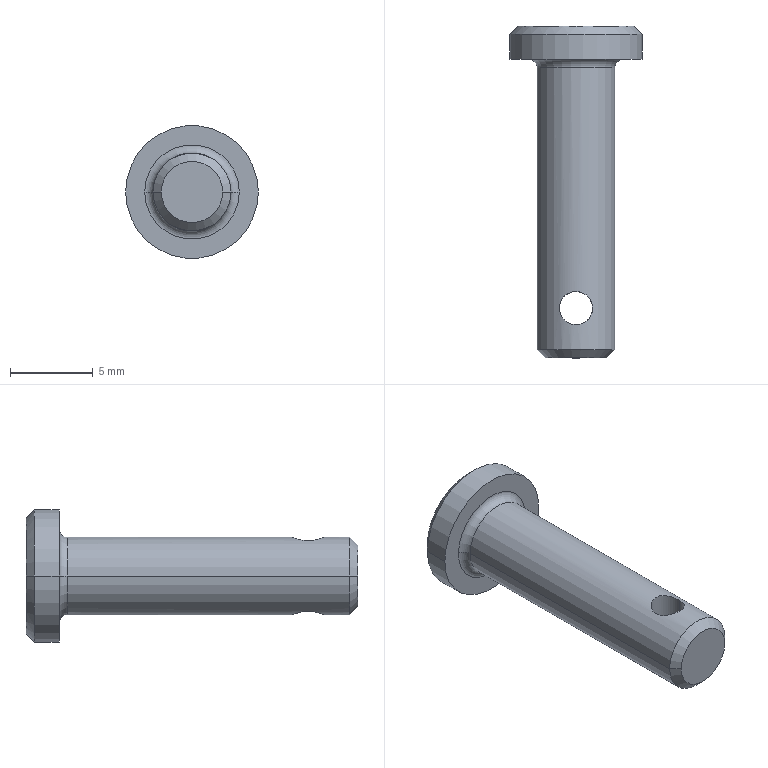Part | SolidWorks | features Chamfer 1, Fillet 1, ICE 1, Revolution 1 | 1 solid | 15 faces | box 8 x 20 x 8 mm | volume 394.503 mm3 | cylinder 6 | cone 4 | plane 3 | torus 2 | commonest cylinder face diameters 2 x2 4.7 x2 8 x2
STEP:
#1=CARTESIAN_POINT('',(1.,-17.,-2.127));
#2=VERTEX_POINT('',#1);
#3=CARTESIAN_POINT('',(-1.,-17.,-2.127));
#4=VERTEX_POINT('',#3);
#5=CARTESIAN_POINT('',(1.,-17.,-2.127));
#6=CARTESIAN_POINT('',(1.,-17.134,-2.127));
#7=CARTESIAN_POINT('',(0.9731,-17.265,-2.14));
#8=CARTESIAN_POINT('',(0.8722,-17.506,-2.183));
#9=CARTESIAN_POINT('',(0.7982,-17.616,-2.212));
#10=CARTESIAN_POINT('',(0.616,-17.798,-2.27));
#11=CARTESIAN_POINT('',(0.5058,-17.872,-2.298));
#12=CARTESIAN_POINT('',(0.2655,-17.973,-2.338));
#13=CARTESIAN_POINT('',(0.1329,-18.,-2.35));
#14=CARTESIAN_POINT('',(-0.1318,-18.,-2.35));
#15=CARTESIAN_POINT('',(-0.2639,-17.974,-2.338));
#16=CARTESIAN_POINT('',(-0.5076,-17.872,-2.298));
#17=CARTESIAN_POINT('',(-0.6167,-17.798,-2.27));
#18=CARTESIAN_POINT('',(-0.7992,-17.615,-2.212));
#19=CARTESIAN_POINT('',(-0.873,-17.505,-2.183));
#20=CARTESIAN_POINT('',(-0.973,-17.265,-2.14));
#21=CARTESIAN_POINT('',(-1.,-17.132,-2.127));
#22=CARTESIAN_POINT('',(-1.,-17.,-2.127));
#23=B_SPLINE_CURVE_WITH_KNOTS('',3,(#5,#6,#7,#8,#9,#10,#11,#12,#13,#14,#15,#16,#17,#18,#19,#20,#21,#22),.UNSPECIFIED.,.F.,.F.,(4,2,2,2,2,2,2,2,4),(0.,0.0003956,0.0007911,0.001187,0.001582,0.001978,0.002373,0.002769,0.003164),.UNSPECIFIED.);
#24=EDGE_CURVE('',#2,#4,#23,.T.);
#25=ORIENTED_EDGE('',*,*,#24,.T.);
#26=CARTESIAN_POINT('',(-1.,-17.,2.127));
#27=VERTEX_POINT('',#26);
#28=CARTESIAN_POINT('',(-1.,-17.,-4.));
#29=DIRECTION('',(0.,0.,1.));
#30=VECTOR('',#29,1000.);
#31=LINE('',#28,#30);
#32=EDGE_CURVE('',#4,#27,#31,.T.);
#33=ORIENTED_EDGE('',*,*,#32,.T.);
#34=CARTESIAN_POINT('',(1.,-17.,2.127));
#35=VERTEX_POINT('',#34);
#36=CARTESIAN_POINT('',(-1.,-17.,2.127));
#37=CARTESIAN_POINT('',(-1.,-17.132,2.127));
#38=CARTESIAN_POINT('',(-0.9733,-17.264,2.14));
#39=CARTESIAN_POINT('',(-0.8723,-17.506,2.183));
#40=CARTESIAN_POINT('',(-0.7988,-17.615,2.212));
#41=CARTESIAN_POINT('',(-0.6151,-17.799,2.27));
#42=CARTESIAN_POINT('',(-0.5058,-17.872,2.298));
#43=CARTESIAN_POINT('',(-0.2646,-17.973,2.338));
#44=CARTESIAN_POINT('',(-0.1321,-18.,2.35));
#45=CARTESIAN_POINT('',(0.1317,-18.,2.35));
#46=CARTESIAN_POINT('',(0.2646,-17.973,2.338));
#47=CARTESIAN_POINT('',(0.5058,-17.872,2.298));
#48=CARTESIAN_POINT('',(0.6155,-17.799,2.27));
#49=CARTESIAN_POINT('',(0.8909,-17.523,2.183));
#50=CARTESIAN_POINT('',(1.,-17.268,2.127));
#51=CARTESIAN_POINT('',(1.,-17.,2.127));
#52=B_SPLINE_CURVE_WITH_KNOTS('',3,(#36,#37,#38,#39,#40,#41,#42,#43,#44,#45,#46,#47,#48,#49,#50,#51),.UNSPECIFIED.,.F.,.F.,(4,2,2,2,2,2,2,4),(0.003164,0.00356,0.003955,0.00435,0.004745,0.00514,0.005536,0.006326),.UNSPECIFIED.);
#53=EDGE_CURVE('',#27,#35,#52,.T.);
#54=ORIENTED_EDGE('',*,*,#53,.T.);
#55=CARTESIAN_POINT('',(1.,-17.,-4.));
#56=DIRECTION('',(0.,0.,1.));
#57=VECTOR('',#56,1000.);
#58=LINE('',#55,#57);
#59=EDGE_CURVE('',#2,#35,#58,.T.);
#60=ORIENTED_EDGE('',*,*,#59,.F.);
#61=EDGE_LOOP('',(#25,#33,#54,#60));
#62=FACE_OUTER_BOUND('',#61,.T.);
#63=CARTESIAN_POINT('',(0.,-17.,-4.));
#64=DIRECTION('',(0.,0.,1.));
#65=DIRECTION('',(1.,0.,0.));
#66=AXIS2_PLACEMENT_3D('',#63,#64,#65);
#67=CYLINDRICAL_SURFACE('',#66,1.);
#68=ADVANCED_FACE('',(#62),#67,.F.);
#69=CARTESIAN_POINT('',(-3.5,0.,0.));
#70=VERTEX_POINT('',#69);
#71=CARTESIAN_POINT('',(3.5,0.,0.));
#72=VERTEX_POINT('',#71);
#73=CARTESIAN_POINT('',(0.,0.,0.));
#74=DIRECTION('',(0.,1.,0.));
#75=DIRECTION('',(-1.,0.,0.));
#76=AXIS2_PLACEMENT_3D('',#73,#74,#75);
#77=CIRCLE('',#76,3.5);
#78=EDGE_CURVE('',#70,#72,#77,.T.);
#79=ORIENTED_EDGE('',*,*,#78,.F.);
#80=CARTESIAN_POINT('',(-4.,-0.5,0.));
#81=VERTEX_POINT('',#80);
#82=CARTESIAN_POINT('',(-4.,-0.5,0.));
#83=DIRECTION('',(-0.7071,-0.7071,0.));
#84=VECTOR('',#83,1000.);
#85=LINE('',#82,#84);
#86=EDGE_CURVE('',#70,#81,#85,.T.);
#87=ORIENTED_EDGE('',*,*,#86,.T.);
#88=CARTESIAN_POINT('',(4.,-0.5,0.));
#89=VERTEX_POINT('',#88);
#90=CARTESIAN_POINT('',(0.,-0.5,0.));
#91=DIRECTION('',(0.,-1.,0.));
#92=DIRECTION('',(-1.,0.,0.));
#93=AXIS2_PLACEMENT_3D('',#90,#91,#92);
#94=CIRCLE('',#93,4.);
#95=EDGE_CURVE('',#89,#81,#94,.T.);
#96=ORIENTED_EDGE('',*,*,#95,.F.);
#97=CARTESIAN_POINT('',(4.,-0.5,0.));
#98=DIRECTION('',(0.7071,-0.7071,0.));
#99=VECTOR('',#98,1000.);
#100=LINE('',#97,#99);
#101=EDGE_CURVE('',#72,#89,#100,.T.);
#102=ORIENTED_EDGE('',*,*,#101,.F.);
#103=EDGE_LOOP('',(#79,#87,#96,#102));
#104=FACE_OUTER_BOUND('',#103,.T.);
#105=CARTESIAN_POINT('',(0.,-0.5,0.));
#106=DIRECTION('',(0.,-1.,0.));
#107=DIRECTION('',(1.,0.,0.));
#108=AXIS2_PLACEMENT_3D('',#105,#106,#107);
#109=CONICAL_SURFACE('',#108,4.,0.7854);
#110=ADVANCED_FACE('',(#104),#109,.T.);
#111=CARTESIAN_POINT('',(1.85,-20.,0.));
#112=VERTEX_POINT('',#111);
#113=CARTESIAN_POINT('',(-1.85,-20.,0.));
#114=VERTEX_POINT('',#113);
#115=CARTESIAN_POINT('',(0.,-20.,0.));
#116=DIRECTION('',(0.,-1.,0.));
#117=DIRECTION('',(1.,0.,0.));
#118=AXIS2_PLACEMENT_3D('',#115,#116,#117);
#119=CIRCLE('',#118,1.85);
#120=EDGE_CURVE('',#112,#114,#119,.T.);
#121=ORIENTED_EDGE('',*,*,#120,.F.);
#122=CARTESIAN_POINT('',(2.35,-19.5,0.));
#123=VERTEX_POINT('',#122);
#124=CARTESIAN_POINT('',(1.85,-20.,0.));
#125=DIRECTION('',(0.7071,0.7071,0.));
#126=VECTOR('',#125,1000.);
#127=LINE('',#124,#126);
#128=EDGE_CURVE('',#112,#123,#127,.T.);
#129=ORIENTED_EDGE('',*,*,#128,.T.);
#130=CARTESIAN_POINT('',(-2.35,-19.5,0.));
#131=VERTEX_POINT('',#130);
#132=CARTESIAN_POINT('',(0.,-19.5,0.));
#133=DIRECTION('',(0.,1.,0.));
#134=DIRECTION('',(1.,0.,0.));
#135=AXIS2_PLACEMENT_3D('',#132,#133,#134);
#136=CIRCLE('',#135,2.35);
#137=EDGE_CURVE('',#131,#123,#136,.T.);
#138=ORIENTED_EDGE('',*,*,#137,.F.);
#139=CARTESIAN_POINT('',(-1.85,-20.,0.));
#140=DIRECTION('',(-0.7071,0.7071,0.));
#141=VECTOR('',#140,1000.);
#142=LINE('',#139,#141);
#143=EDGE_CURVE('',#114,#131,#142,.T.);
#144=ORIENTED_EDGE('',*,*,#143,.F.);
#145=EDGE_LOOP('',(#121,#129,#138,#144));
#146=FACE_OUTER_BOUND('',#145,.T.);
#147=CARTESIAN_POINT('',(0.,-20.,0.));
#148=DIRECTION('',(0.,1.,0.));
#149=DIRECTION('',(-1.,0.,0.));
#150=AXIS2_PLACEMENT_3D('',#147,#148,#149);
#151=CONICAL_SURFACE('',#150,1.85,0.7854);
#152=ADVANCED_FACE('',(#146),#151,.T.);
#153=CARTESIAN_POINT('',(-2.35,-2.5,0.));
#154=VERTEX_POINT('',#153);
#155=CARTESIAN_POINT('',(2.35,-2.5,0.));
#156=VERTEX_POINT('',#155);
#157=CARTESIAN_POINT('',(0.,-2.5,0.));
#158=DIRECTION('',(0.,-1.,0.));
#159=DIRECTION('',(1.,0.,0.));
#160=AXIS2_PLACEMENT_3D('',#157,#158,#159);
#161=CIRCLE('',#160,2.35);
#162=EDGE_CURVE('',#154,#156,#161,.T.);
#163=ORIENTED_EDGE('',*,*,#162,.F.);
#164=CARTESIAN_POINT('',(-2.85,-2.,0.));
#165=VERTEX_POINT('',#164);
#166=CARTESIAN_POINT('',(-2.85,-2.5,0.));
#167=DIRECTION('',(0.,0.,1.));
#168=DIRECTION('',(1.,0.,0.));
#169=AXIS2_PLACEMENT_3D('',#166,#167,#168);
#170=CIRCLE('',#169,0.5);
#171=EDGE_CURVE('',#154,#165,#170,.T.);
#172=ORIENTED_EDGE('',*,*,#171,.T.);
#173=CARTESIAN_POINT('',(2.85,-2.,0.));
#174=VERTEX_POINT('',#173);
#175=CARTESIAN_POINT('',(0.,-2.,0.));
#176=DIRECTION('',(0.,1.,0.));
#177=DIRECTION('',(1.,0.,0.));
#178=AXIS2_PLACEMENT_3D('',#175,#176,#177);
#179=CIRCLE('',#178,2.85);
#180=EDGE_CURVE('',#174,#165,#179,.T.);
#181=ORIENTED_EDGE('',*,*,#180,.F.);
#182=CARTESIAN_POINT('',(2.85,-2.5,0.));
#183=DIRECTION('',(0.,0.,-1.));
#184=DIRECTION('',(-1.,0.,0.));
#185=AXIS2_PLACEMENT_3D('',#182,#183,#184);
#186=CIRCLE('',#185,0.5);
#187=EDGE_CURVE('',#156,#174,#186,.T.);
#188=ORIENTED_EDGE('',*,*,#187,.F.);
#189=EDGE_LOOP('',(#163,#172,#181,#188));
#190=FACE_OUTER_BOUND('',#189,.T.);
#191=CARTESIAN_POINT('',(0.,-2.5,0.));
#192=DIRECTION('',(0.,-1.,0.));
#193=DIRECTION('',(1.,0.,0.));
#194=AXIS2_PLACEMENT_3D('',#191,#192,#193);
#195=TOROIDAL_SURFACE('',#194,2.85,0.5);
#196=ADVANCED_FACE('',(#190),#195,.F.);
#197=CARTESIAN_POINT('',(1.,-17.,2.127));
#198=CARTESIAN_POINT('',(1.,-16.866,2.127));
#199=CARTESIAN_POINT('',(0.9731,-16.735,2.14));
#200=CARTESIAN_POINT('',(0.8722,-16.494,2.183));
#201=CARTESIAN_POINT('',(0.7982,-16.384,2.212));
#202=CARTESIAN_POINT('',(0.616,-16.202,2.27));
#203=CARTESIAN_POINT('',(0.5058,-16.128,2.298));
#204=CARTESIAN_POINT('',(0.2655,-16.027,2.338));
#205=CARTESIAN_POINT('',(0.1329,-16.,2.35));
#206=CARTESIAN_POINT('',(-0.1318,-16.,2.35));
#207=CARTESIAN_POINT('',(-0.2639,-16.026,2.338));
#208=CARTESIAN_POINT('',(-0.5076,-16.128,2.298));
#209=CARTESIAN_POINT('',(-0.6167,-16.202,2.27));
#210=CARTESIAN_POINT('',(-0.7992,-16.385,2.212));
#211=CARTESIAN_POINT('',(-0.873,-16.495,2.183));
#212=CARTESIAN_POINT('',(-0.973,-16.735,2.14));
#213=CARTESIAN_POINT('',(-1.,-16.868,2.127));
#214=CARTESIAN_POINT('',(-1.,-17.,2.127));
#215=B_SPLINE_CURVE_WITH_KNOTS('',3,(#197,#198,#199,#200,#201,#202,#203,#204,#205,#206,#207,#208,#209,#210,#211,#212,#213,#214),.UNSPECIFIED.,.F.,.F.,(4,2,2,2,2,2,2,2,4),(0.,0.0003956,0.0007911,0.001187,0.001582,0.001978,0.002373,0.002769,0.003164),.UNSPECIFIED.);
#216=EDGE_CURVE('',#35,#27,#215,.T.);
#217=ORIENTED_EDGE('',*,*,#216,.F.);
#218=ORIENTED_EDGE('',*,*,#53,.F.);
#219=EDGE_LOOP('',(#217,#218));
#220=FACE_BOUND('',#219,.T.);
#221=CARTESIAN_POINT('',(0.,-2.5,0.));
#222=DIRECTION('',(0.,-1.,0.));
#223=DIRECTION('',(1.,0.,0.));
#224=AXIS2_PLACEMENT_3D('',#221,#222,#223);
#225=CIRCLE('',#224,2.35);
#226=EDGE_CURVE('',#156,#154,#225,.T.);
#227=ORIENTED_EDGE('',*,*,#226,.T.);
#228=CARTESIAN_POINT('',(-2.35,-273.134,0.));
#229=DIRECTION('',(0.,-1.,0.));
#230=VECTOR('',#229,1000.);
#231=LINE('',#228,#230);
#232=EDGE_CURVE('',#154,#131,#231,.T.);
#233=ORIENTED_EDGE('',*,*,#232,.T.);
#234=ORIENTED_EDGE('',*,*,#137,.T.);
#235=CARTESIAN_POINT('',(2.35,-273.134,0.));
#236=DIRECTION('',(0.,-1.,0.));
#237=VECTOR('',#236,1000.);
#238=LINE('',#235,#237);
#239=EDGE_CURVE('',#156,#123,#238,.T.);
#240=ORIENTED_EDGE('',*,*,#239,.F.);
#241=EDGE_LOOP('',(#227,#233,#234,#240));
#242=FACE_OUTER_BOUND('',#241,.T.);
#243=CARTESIAN_POINT('',(0.,-273.134,0.));
#244=DIRECTION('',(0.,-1.,0.));
#245=DIRECTION('',(1.,0.,0.));
#246=AXIS2_PLACEMENT_3D('',#243,#244,#245);
#247=CYLINDRICAL_SURFACE('',#246,2.35);
#248=ADVANCED_FACE('',(#220,#242),#247,.T.);
#249=ORIENTED_EDGE('',*,*,#95,.T.);
#250=CARTESIAN_POINT('',(-4.,-2.,0.));
#251=VERTEX_POINT('',#250);
#252=CARTESIAN_POINT('',(-4.,-273.134,0.));
#253=DIRECTION('',(0.,-1.,0.));
#254=VECTOR('',#253,1000.);
#255=LINE('',#252,#254);
#256=EDGE_CURVE('',#81,#251,#255,.T.);
#257=ORIENTED_EDGE('',*,*,#256,.T.);
#258=CARTESIAN_POINT('',(4.,-2.,0.));
#259=VERTEX_POINT('',#258);
#260=CARTESIAN_POINT('',(0.,-2.,0.));
#261=DIRECTION('',(0.,-1.,0.));
#262=DIRECTION('',(1.,0.,0.));
#263=AXIS2_PLACEMENT_3D('',#260,#261,#262);
#264=CIRCLE('',#263,4.);
#265=EDGE_CURVE('',#259,#251,#264,.T.);
#266=ORIENTED_EDGE('',*,*,#265,.F.);
#267=CARTESIAN_POINT('',(4.,-273.134,0.));
#268=DIRECTION('',(0.,-1.,0.));
#269=VECTOR('',#268,1000.);
#270=LINE('',#267,#269);
#271=EDGE_CURVE('',#89,#259,#270,.T.);
#272=ORIENTED_EDGE('',*,*,#271,.F.);
#273=EDGE_LOOP('',(#249,#257,#266,#272));
#274=FACE_OUTER_BOUND('',#273,.T.);
#275=CARTESIAN_POINT('',(0.,-273.134,0.));
#276=DIRECTION('',(0.,-1.,0.));
#277=DIRECTION('',(1.,0.,0.));
#278=AXIS2_PLACEMENT_3D('',#275,#276,#277);
#279=CYLINDRICAL_SURFACE('',#278,4.);
#280=ADVANCED_FACE('',(#274),#279,.T.);
#281=CARTESIAN_POINT('',(0.,0.,0.));
#282=DIRECTION('',(0.,1.,0.));
#283=DIRECTION('',(-1.,0.,0.));
#284=AXIS2_PLACEMENT_3D('',#281,#282,#283);
#285=CIRCLE('',#284,3.5);
#286=EDGE_CURVE('',#72,#70,#285,.T.);
#287=ORIENTED_EDGE('',*,*,#286,.T.);
#288=ORIENTED_EDGE('',*,*,#78,.T.);
#289=EDGE_LOOP('',(#287,#288));
#290=FACE_OUTER_BOUND('',#289,.T.);
#291=CARTESIAN_POINT('',(0.,0.,0.));
#292=DIRECTION('',(0.,1.,0.));
#293=DIRECTION('',(-1.,0.,0.));
#294=AXIS2_PLACEMENT_3D('',#291,#292,#293);
#295=PLANE('',#294);
#296=ADVANCED_FACE('',(#290),#295,.T.);
#297=ORIENTED_EDGE('',*,*,#256,.F.);
#298=CARTESIAN_POINT('',(0.,-0.5,0.));
#299=DIRECTION('',(0.,-1.,0.));
#300=DIRECTION('',(-1.,0.,0.));
#301=AXIS2_PLACEMENT_3D('',#298,#299,#300);
#302=CIRCLE('',#301,4.);
#303=EDGE_CURVE('',#81,#89,#302,.T.);
#304=ORIENTED_EDGE('',*,*,#303,.T.);
#305=ORIENTED_EDGE('',*,*,#271,.T.);
#306=CARTESIAN_POINT('',(0.,-2.,0.));
#307=DIRECTION('',(0.,-1.,0.));
#308=DIRECTION('',(1.,0.,0.));
#309=AXIS2_PLACEMENT_3D('',#306,#307,#308);
#310=CIRCLE('',#309,4.);
#311=EDGE_CURVE('',#251,#259,#310,.T.);
#312=ORIENTED_EDGE('',*,*,#311,.F.);
#313=EDGE_LOOP('',(#297,#304,#305,#312));
#314=FACE_OUTER_BOUND('',#313,.T.);
#315=CARTESIAN_POINT('',(0.,-273.134,0.));
#316=DIRECTION('',(0.,-1.,0.));
#317=DIRECTION('',(1.,0.,0.));
#318=AXIS2_PLACEMENT_3D('',#315,#316,#317);
#319=CYLINDRICAL_SURFACE('',#318,4.);
#320=ADVANCED_FACE('',(#314),#319,.T.);
#321=ORIENTED_EDGE('',*,*,#180,.T.);
#322=CARTESIAN_POINT('',(0.,-2.,0.));
#323=DIRECTION('',(0.,1.,0.));
#324=DIRECTION('',(1.,0.,0.));
#325=AXIS2_PLACEMENT_3D('',#322,#323,#324);
#326=CIRCLE('',#325,2.85);
#327=EDGE_CURVE('',#165,#174,#326,.T.);
#328=ORIENTED_EDGE('',*,*,#327,.T.);
#329=EDGE_LOOP('',(#321,#328));
#330=FACE_BOUND('',#329,.T.);
#331=ORIENTED_EDGE('',*,*,#265,.T.);
#332=ORIENTED_EDGE('',*,*,#311,.T.);
#333=EDGE_LOOP('',(#331,#332));
#334=FACE_OUTER_BOUND('',#333,.T.);
#335=CARTESIAN_POINT('',(4.,-2.,0.));
#336=DIRECTION('',(0.,-1.,0.));
#337=DIRECTION('',(1.,0.,0.));
#338=AXIS2_PLACEMENT_3D('',#335,#336,#337);
#339=PLANE('',#338);
#340=ADVANCED_FACE('',(#330,#334),#339,.T.);
#341=ORIENTED_EDGE('',*,*,#232,.F.);
#342=ORIENTED_EDGE('',*,*,#162,.T.);
#343=ORIENTED_EDGE('',*,*,#239,.T.);
#344=CARTESIAN_POINT('',(0.,-19.5,0.));
#345=DIRECTION('',(0.,1.,0.));
#346=DIRECTION('',(1.,0.,0.));
#347=AXIS2_PLACEMENT_3D('',#344,#345,#346);
#348=CIRCLE('',#347,2.35);
#349=EDGE_CURVE('',#123,#131,#348,.T.);
#350=ORIENTED_EDGE('',*,*,#349,.T.);
#351=EDGE_LOOP('',(#341,#342,#343,#350));
#352=FACE_OUTER_BOUND('',#351,.T.);
#353=ORIENTED_EDGE('',*,*,#24,.F.);
#354=CARTESIAN_POINT('',(-1.,-17.,-2.127));
#355=CARTESIAN_POINT('',(-1.,-16.868,-2.127));
#356=CARTESIAN_POINT('',(-0.9733,-16.736,-2.14));
#357=CARTESIAN_POINT('',(-0.8723,-16.494,-2.183));
#358=CARTESIAN_POINT('',(-0.7988,-16.385,-2.212));
#359=CARTESIAN_POINT('',(-0.6151,-16.201,-2.27));
#360=CARTESIAN_POINT('',(-0.5058,-16.128,-2.298));
#361=CARTESIAN_POINT('',(-0.2646,-16.027,-2.338));
#362=CARTESIAN_POINT('',(-0.1321,-16.,-2.35));
#363=CARTESIAN_POINT('',(0.1317,-16.,-2.35));
#364=CARTESIAN_POINT('',(0.2646,-16.027,-2.338));
#365=CARTESIAN_POINT('',(0.5058,-16.128,-2.298));
#366=CARTESIAN_POINT('',(0.6155,-16.201,-2.27));
#367=CARTESIAN_POINT('',(0.8909,-16.477,-2.183));
#368=CARTESIAN_POINT('',(1.,-16.732,-2.127));
#369=CARTESIAN_POINT('',(1.,-17.,-2.127));
#370=B_SPLINE_CURVE_WITH_KNOTS('',3,(#354,#355,#356,#357,#358,#359,#360,#361,#362,#363,#364,#365,#366,#367,#368,#369),.UNSPECIFIED.,.F.,.F.,(4,2,2,2,2,2,2,4),(0.003164,0.00356,0.003955,0.00435,0.004745,0.00514,0.005536,0.006326),.UNSPECIFIED.);
#371=EDGE_CURVE('',#4,#2,#370,.T.);
#372=ORIENTED_EDGE('',*,*,#371,.F.);
#373=EDGE_LOOP('',(#353,#372));
#374=FACE_BOUND('',#373,.T.);
#375=CARTESIAN_POINT('',(0.,-273.134,0.));
#376=DIRECTION('',(0.,-1.,0.));
#377=DIRECTION('',(1.,0.,0.));
#378=AXIS2_PLACEMENT_3D('',#375,#376,#377);
#379=CYLINDRICAL_SURFACE('',#378,2.35);
#380=ADVANCED_FACE('',(#352,#374),#379,.T.);
#381=CARTESIAN_POINT('',(0.,-20.,0.));
#382=DIRECTION('',(0.,-1.,0.));
#383=DIRECTION('',(1.,0.,0.));
#384=AXIS2_PLACEMENT_3D('',#381,#382,#383);
#385=CIRCLE('',#384,1.85);
#386=EDGE_CURVE('',#114,#112,#385,.T.);
#387=ORIENTED_EDGE('',*,*,#386,.T.);
#388=ORIENTED_EDGE('',*,*,#120,.T.);
#389=EDGE_LOOP('',(#387,#388));
#390=FACE_OUTER_BOUND('',#389,.T.);
#391=CARTESIAN_POINT('',(2.35,-20.,0.));
#392=DIRECTION('',(0.,-1.,0.));
#393=DIRECTION('',(1.,0.,0.));
#394=AXIS2_PLACEMENT_3D('',#391,#392,#393);
#395=PLANE('',#394);
#396=ADVANCED_FACE('',(#390),#395,.T.);
#397=ORIENTED_EDGE('',*,*,#171,.F.);
#398=ORIENTED_EDGE('',*,*,#226,.F.);
#399=ORIENTED_EDGE('',*,*,#187,.T.);
#400=ORIENTED_EDGE('',*,*,#327,.F.);
#401=EDGE_LOOP('',(#397,#398,#399,#400));
#402=FACE_OUTER_BOUND('',#401,.T.);
#403=CARTESIAN_POINT('',(0.,-2.5,0.));
#404=DIRECTION('',(0.,-1.,0.));
#405=DIRECTION('',(1.,0.,0.));
#406=AXIS2_PLACEMENT_3D('',#403,#404,#405);
#407=TOROIDAL_SURFACE('',#406,2.85,0.5);
#408=ADVANCED_FACE('',(#402),#407,.F.);
#409=ORIENTED_EDGE('',*,*,#128,.F.);
#410=ORIENTED_EDGE('',*,*,#386,.F.);
#411=ORIENTED_EDGE('',*,*,#143,.T.);
#412=ORIENTED_EDGE('',*,*,#349,.F.);
#413=EDGE_LOOP('',(#409,#410,#411,#412));
#414=FACE_OUTER_BOUND('',#413,.T.);
#415=CARTESIAN_POINT('',(0.,-20.,0.));
#416=DIRECTION('',(0.,1.,0.));
#417=DIRECTION('',(-1.,0.,0.));
#418=AXIS2_PLACEMENT_3D('',#415,#416,#417);
#419=CONICAL_SURFACE('',#418,1.85,0.7854);
#420=ADVANCED_FACE('',(#414),#419,.T.);
#421=ORIENTED_EDGE('',*,*,#86,.F.);
#422=ORIENTED_EDGE('',*,*,#286,.F.);
#423=ORIENTED_EDGE('',*,*,#101,.T.);
#424=ORIENTED_EDGE('',*,*,#303,.F.);
#425=EDGE_LOOP('',(#421,#422,#423,#424));
#426=FACE_OUTER_BOUND('',#425,.T.);
#427=CARTESIAN_POINT('',(0.,-0.5,0.));
#428=DIRECTION('',(0.,-1.,0.));
#429=DIRECTION('',(1.,0.,0.));
#430=AXIS2_PLACEMENT_3D('',#427,#428,#429);
#431=CONICAL_SURFACE('',#430,4.,0.7854);
#432=ADVANCED_FACE('',(#426),#431,.T.);
#433=ORIENTED_EDGE('',*,*,#32,.F.);
#434=ORIENTED_EDGE('',*,*,#371,.T.);
#435=ORIENTED_EDGE('',*,*,#59,.T.);
#436=ORIENTED_EDGE('',*,*,#216,.T.);
#437=EDGE_LOOP('',(#433,#434,#435,#436));
#438=FACE_OUTER_BOUND('',#437,.T.);
#439=CARTESIAN_POINT('',(0.,-17.,-4.));
#440=DIRECTION('',(0.,0.,1.));
#441=DIRECTION('',(1.,0.,0.));
#442=AXIS2_PLACEMENT_3D('',#439,#440,#441);
#443=CYLINDRICAL_SURFACE('',#442,1.);
#444=ADVANCED_FACE('',(#438),#443,.F.);
#445=CLOSED_SHELL('',(#68,#110,#152,#196,#248,#280,#296,#320,#340,#380,#396,#408,#420,#432,#444));
#446=MANIFOLD_SOLID_BREP('',#445);
#447=CARTESIAN_POINT('',(0.,0.,0.));
#448=DIRECTION('',(0.,0.,1.));
#449=DIRECTION('',(1.,0.,0.));
#450=AXIS2_PLACEMENT_3D('',#447,#448,#449);
#451=(LENGTH_UNIT()NAMED_UNIT(*)SI_UNIT(.MILLI.,.METRE.));
#452=UNCERTAINTY_MEASURE_WITH_UNIT(LENGTH_MEASURE(0.00001),#451,'','');
#453=(NAMED_UNIT(*)PLANE_ANGLE_UNIT()SI_UNIT($,.RADIAN.));
#454=(NAMED_UNIT(*)SI_UNIT($,.STERADIAN.)SOLID_ANGLE_UNIT());
#455=(GEOMETRIC_REPRESENTATION_CONTEXT(3)GLOBAL_UNCERTAINTY_ASSIGNED_CONTEXT((#452))GLOBAL_UNIT_ASSIGNED_CONTEXT((#451,#453,#454))REPRESENTATION_CONTEXT('',''));
#456=ADVANCED_BREP_SHAPE_REPRESENTATION('',(#446,#450),#455);